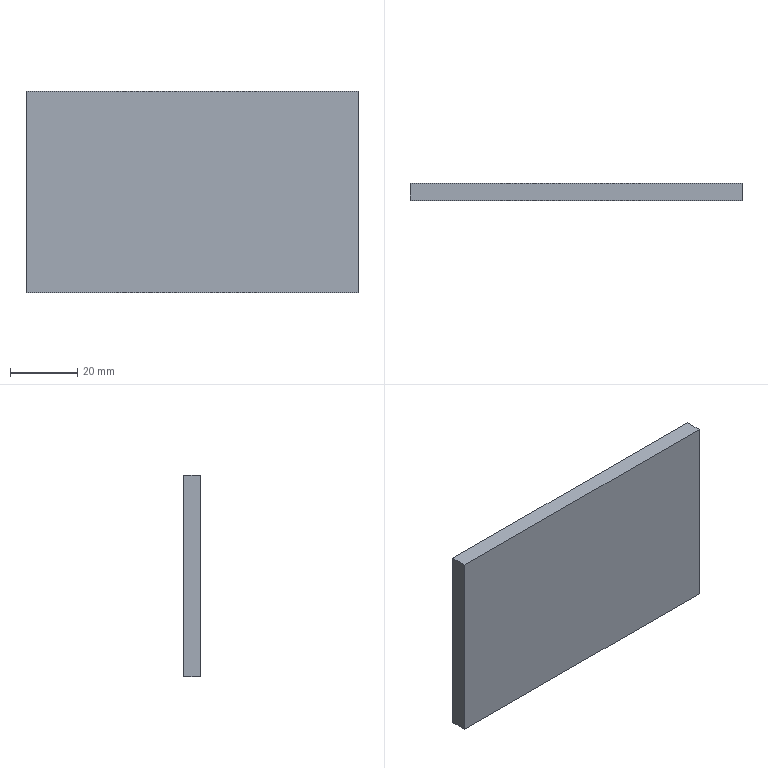Part | SolidWorks | features Extrusion 1 | 1 solid | 6 faces | box 99 x 5 x 60 mm | volume 29700 mm3 | plane 6
STEP:
#1=CARTESIAN_POINT('',(49.5,-2.5,-30.));
#2=VERTEX_POINT('',#1);
#3=CARTESIAN_POINT('',(49.5,2.5,-30.));
#4=VERTEX_POINT('',#3);
#5=CARTESIAN_POINT('',(49.5,-2.5,-30.));
#6=DIRECTION('',(0.,1.,0.));
#7=VECTOR('',#6,1000.);
#8=LINE('',#5,#7);
#9=EDGE_CURVE('',#2,#4,#8,.T.);
#10=ORIENTED_EDGE('',*,*,#9,.T.);
#11=CARTESIAN_POINT('',(49.5,2.5,30.));
#12=VERTEX_POINT('',#11);
#13=CARTESIAN_POINT('',(49.5,2.5,30.));
#14=DIRECTION('',(0.,0.,-1.));
#15=VECTOR('',#14,1000.);
#16=LINE('',#13,#15);
#17=EDGE_CURVE('',#12,#4,#16,.T.);
#18=ORIENTED_EDGE('',*,*,#17,.F.);
#19=CARTESIAN_POINT('',(49.5,-2.5,30.));
#20=VERTEX_POINT('',#19);
#21=CARTESIAN_POINT('',(49.5,-2.5,30.));
#22=DIRECTION('',(0.,1.,0.));
#23=VECTOR('',#22,1000.);
#24=LINE('',#21,#23);
#25=EDGE_CURVE('',#20,#12,#24,.T.);
#26=ORIENTED_EDGE('',*,*,#25,.F.);
#27=CARTESIAN_POINT('',(49.5,-2.5,30.));
#28=DIRECTION('',(0.,0.,-1.));
#29=VECTOR('',#28,1000.);
#30=LINE('',#27,#29);
#31=EDGE_CURVE('',#20,#2,#30,.T.);
#32=ORIENTED_EDGE('',*,*,#31,.T.);
#33=EDGE_LOOP('',(#10,#18,#26,#32));
#34=FACE_OUTER_BOUND('',#33,.T.);
#35=CARTESIAN_POINT('',(49.5,-2.5,30.));
#36=DIRECTION('',(-1.,0.,0.));
#37=DIRECTION('',(0.,0.,1.));
#38=AXIS2_PLACEMENT_3D('',#35,#36,#37);
#39=PLANE('',#38);
#40=ADVANCED_FACE('',(#34),#39,.F.);
#41=CARTESIAN_POINT('',(-49.5,2.5,-30.));
#42=VERTEX_POINT('',#41);
#43=CARTESIAN_POINT('',(-49.5,2.5,-30.));
#44=DIRECTION('',(-1.,0.,0.));
#45=VECTOR('',#44,1000.);
#46=LINE('',#43,#45);
#47=EDGE_CURVE('',#4,#42,#46,.T.);
#48=ORIENTED_EDGE('',*,*,#47,.T.);
#49=CARTESIAN_POINT('',(-49.5,2.5,30.));
#50=VERTEX_POINT('',#49);
#51=CARTESIAN_POINT('',(-49.5,2.5,30.));
#52=DIRECTION('',(0.,0.,-1.));
#53=VECTOR('',#52,1000.);
#54=LINE('',#51,#53);
#55=EDGE_CURVE('',#50,#42,#54,.T.);
#56=ORIENTED_EDGE('',*,*,#55,.F.);
#57=CARTESIAN_POINT('',(-49.5,2.5,30.));
#58=DIRECTION('',(-1.,0.,0.));
#59=VECTOR('',#58,1000.);
#60=LINE('',#57,#59);
#61=EDGE_CURVE('',#12,#50,#60,.T.);
#62=ORIENTED_EDGE('',*,*,#61,.F.);
#63=ORIENTED_EDGE('',*,*,#17,.T.);
#64=EDGE_LOOP('',(#48,#56,#62,#63));
#65=FACE_OUTER_BOUND('',#64,.T.);
#66=CARTESIAN_POINT('',(-49.5,2.5,30.));
#67=DIRECTION('',(0.,-1.,0.));
#68=DIRECTION('',(0.,0.,-1.));
#69=AXIS2_PLACEMENT_3D('',#66,#67,#68);
#70=PLANE('',#69);
#71=ADVANCED_FACE('',(#65),#70,.F.);
#72=CARTESIAN_POINT('',(-49.5,-2.5,-30.));
#73=VERTEX_POINT('',#72);
#74=CARTESIAN_POINT('',(-49.5,-2.5,-30.));
#75=DIRECTION('',(0.,-1.,0.));
#76=VECTOR('',#75,1000.);
#77=LINE('',#74,#76);
#78=EDGE_CURVE('',#42,#73,#77,.T.);
#79=ORIENTED_EDGE('',*,*,#78,.T.);
#80=CARTESIAN_POINT('',(-49.5,-2.5,30.));
#81=VERTEX_POINT('',#80);
#82=CARTESIAN_POINT('',(-49.5,-2.5,30.));
#83=DIRECTION('',(0.,0.,-1.));
#84=VECTOR('',#83,1000.);
#85=LINE('',#82,#84);
#86=EDGE_CURVE('',#81,#73,#85,.T.);
#87=ORIENTED_EDGE('',*,*,#86,.F.);
#88=CARTESIAN_POINT('',(-49.5,-2.5,30.));
#89=DIRECTION('',(0.,-1.,0.));
#90=VECTOR('',#89,1000.);
#91=LINE('',#88,#90);
#92=EDGE_CURVE('',#50,#81,#91,.T.);
#93=ORIENTED_EDGE('',*,*,#92,.F.);
#94=ORIENTED_EDGE('',*,*,#55,.T.);
#95=EDGE_LOOP('',(#79,#87,#93,#94));
#96=FACE_OUTER_BOUND('',#95,.T.);
#97=CARTESIAN_POINT('',(-49.5,-2.5,30.));
#98=DIRECTION('',(1.,0.,0.));
#99=DIRECTION('',(0.,0.,-1.));
#100=AXIS2_PLACEMENT_3D('',#97,#98,#99);
#101=PLANE('',#100);
#102=ADVANCED_FACE('',(#96),#101,.F.);
#103=CARTESIAN_POINT('',(-49.5,-2.5,-30.));
#104=DIRECTION('',(1.,0.,0.));
#105=VECTOR('',#104,1000.);
#106=LINE('',#103,#105);
#107=EDGE_CURVE('',#73,#2,#106,.T.);
#108=ORIENTED_EDGE('',*,*,#107,.T.);
#109=ORIENTED_EDGE('',*,*,#31,.F.);
#110=CARTESIAN_POINT('',(-49.5,-2.5,30.));
#111=DIRECTION('',(1.,0.,0.));
#112=VECTOR('',#111,1000.);
#113=LINE('',#110,#112);
#114=EDGE_CURVE('',#81,#20,#113,.T.);
#115=ORIENTED_EDGE('',*,*,#114,.F.);
#116=ORIENTED_EDGE('',*,*,#86,.T.);
#117=EDGE_LOOP('',(#108,#109,#115,#116));
#118=FACE_OUTER_BOUND('',#117,.T.);
#119=CARTESIAN_POINT('',(-49.5,-2.5,30.));
#120=DIRECTION('',(0.,1.,0.));
#121=DIRECTION('',(0.,0.,1.));
#122=AXIS2_PLACEMENT_3D('',#119,#120,#121);
#123=PLANE('',#122);
#124=ADVANCED_FACE('',(#118),#123,.F.);
#125=ORIENTED_EDGE('',*,*,#25,.T.);
#126=ORIENTED_EDGE('',*,*,#61,.T.);
#127=ORIENTED_EDGE('',*,*,#92,.T.);
#128=ORIENTED_EDGE('',*,*,#114,.T.);
#129=EDGE_LOOP('',(#125,#126,#127,#128));
#130=FACE_OUTER_BOUND('',#129,.T.);
#131=CARTESIAN_POINT('',(0.,0.,30.));
#132=DIRECTION('',(0.,0.,-1.));
#133=DIRECTION('',(-1.,0.,0.));
#134=AXIS2_PLACEMENT_3D('',#131,#132,#133);
#135=PLANE('',#134);
#136=ADVANCED_FACE('',(#130),#135,.F.);
#137=ORIENTED_EDGE('',*,*,#9,.F.);
#138=ORIENTED_EDGE('',*,*,#107,.F.);
#139=ORIENTED_EDGE('',*,*,#78,.F.);
#140=ORIENTED_EDGE('',*,*,#47,.F.);
#141=EDGE_LOOP('',(#137,#138,#139,#140));
#142=FACE_OUTER_BOUND('',#141,.T.);
#143=CARTESIAN_POINT('',(0.,0.,-30.));
#144=DIRECTION('',(0.,0.,-1.));
#145=DIRECTION('',(-1.,0.,0.));
#146=AXIS2_PLACEMENT_3D('',#143,#144,#145);
#147=PLANE('',#146);
#148=ADVANCED_FACE('',(#142),#147,.T.);
#149=CLOSED_SHELL('',(#40,#71,#102,#124,#136,#148));
#150=MANIFOLD_SOLID_BREP('',#149);
#151=CARTESIAN_POINT('',(0.,0.,0.));
#152=DIRECTION('',(0.,0.,1.));
#153=DIRECTION('',(1.,0.,0.));
#154=AXIS2_PLACEMENT_3D('',#151,#152,#153);
#155=(LENGTH_UNIT()NAMED_UNIT(*)SI_UNIT(.MILLI.,.METRE.));
#156=UNCERTAINTY_MEASURE_WITH_UNIT(LENGTH_MEASURE(0.00001),#155,'','');
#157=(NAMED_UNIT(*)PLANE_ANGLE_UNIT()SI_UNIT($,.RADIAN.));
#158=(NAMED_UNIT(*)SI_UNIT($,.STERADIAN.)SOLID_ANGLE_UNIT());
#159=(GEOMETRIC_REPRESENTATION_CONTEXT(3)GLOBAL_UNCERTAINTY_ASSIGNED_CONTEXT((#156))GLOBAL_UNIT_ASSIGNED_CONTEXT((#155,#157,#158))REPRESENTATION_CONTEXT('',''));
#160=ADVANCED_BREP_SHAPE_REPRESENTATION('',(#150,#154),#159);